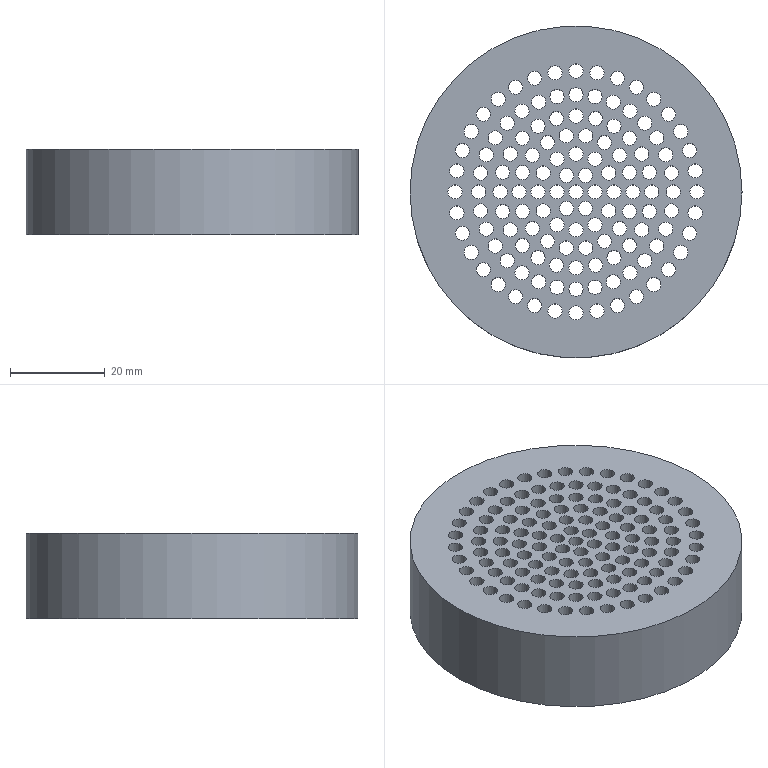NC program | NX | posted with a generic post | part box 70 x 70 x 18 mm
Whole program:
N10 G17 G21 G94 G90
(DRILLING_COPY_2 , TOOL : ZXZ)
N12 T01 M6
N14 G54
N16 G17 G0 G90 X-14.496 Y-14.496 S3000 M3
N18 G43 Z30. H1
N20 G94 G81 G98 Z-1. F250. R3.
N22 X-17.045 Y-11.389
N24 X-18.94 Y-7.845
N26 X-20.106 Y-3.999
N28 X-20.5 Y0.
N30 X-20.106 Y3.999
N32 X-18.94 Y7.845
N34 X-17.045 Y11.389
N36 X-14.496 Y14.496
N38 X-11.389 Y17.045
N40 X-7.845 Y18.94
N42 X-3.999 Y20.106
N44 X0. Y20.5
N46 X3.999 Y20.106
N48 X7.845 Y18.94
N50 X11.389 Y17.045
N52 X14.496 Y14.496
N54 X17.045 Y11.389
N56 X18.94 Y7.845
N58 X20.106 Y3.999
N60 X20.5 Y0.
N62 X20.106 Y-3.999
N64 X18.94 Y-7.845
N66 X17.045 Y-11.389
N68 X14.496 Y-14.496
N70 X11.389 Y-17.045
N72 X7.845 Y-18.94
N74 X3.999 Y-20.106
N76 X0. Y-20.5
N78 X-3.999 Y-20.106
N80 X-7.845 Y-18.94
N82 X-11.389 Y-17.045
N84 X-8. Y-13.856
N86 X-6. Y-10.392
N88 X-4. Y-6.928
N90 X-2. Y-3.464
N92 X-4. Y0.
N94 X-2. Y3.464
N96 X2.
N98 X4. Y6.928
N100 X6. Y10.392
N102 X9.193 Y7.713
N104 X6.928 Y4.
N106 X11.276 Y4.104
N108 X12. Y0.
N110 X11.276 Y-4.104
N112 X9.193 Y-7.713
N114 X6.928 Y-4.
N116 X8. Y0.
N118 X4.
N120 X0.
N122 X2. Y-3.464
N124 X4. Y-6.928
N126 X0. Y-8.
N128 X-2.084 Y-11.818
N130 X-4.141 Y-15.455
N132 X0. Y-16.
N134 X4.141 Y-15.455
N136 X2.084 Y-11.818
N138 X6. Y-10.392
N140 X8. Y-13.856
N142 X11.314 Y-11.314
N144 X13.856 Y-8.
N146 X15.455 Y-4.141
N148 X16. Y0.
N150 X15.455 Y4.141
N152 X13.856 Y8.
N154 X11.314 Y11.314
N156 X8. Y13.856
N158 X4.141 Y15.455
N160 X0. Y16.
N162 X-4.141 Y15.455
N164 X-8. Y13.856
N166 X-6. Y10.392
N168 X-2.084 Y11.818
N170 X2.084
N172 X0. Y8.
N174 X-4. Y6.928
N176 X-6.928 Y4.
N178 X-11.276 Y4.104
N180 X-9.193 Y7.713
N182 X-11.314 Y11.314
N184 X-13.856 Y8.
N186 X-15.455 Y4.141
N188 X-16. Y0.
N190 X-12.
N192 X-8.
N194 X-6.928 Y-4.
N196 X-9.193 Y-7.713
N198 X-11.276 Y-4.104
N200 X-15.455 Y-4.141
N202 X-13.856 Y-8.
N204 X-11.314 Y-11.314
N206 G80
N208 G0 X-11.314 Y-11.314 Z30.
N210 M5
(DRILLING_COPY_COPY , TOOL : 2.5ZT)
N212 T12 M6
N214 G54
N216 G17 G0 G90 X-14.496 Y-14.496 S2971 M3
N218 G43 Z30. H12
N220 G94 G83 G98 Z-19.751 F120. Q2. R3.
N222 X-17.045 Y-11.389
N224 X-18.94 Y-7.845
N226 X-20.106 Y-3.999
N228 X-20.5 Y0.
N230 X-20.106 Y3.999
N232 X-18.94 Y7.845
N234 X-17.045 Y11.389
N236 X-14.496 Y14.496
N238 X-11.389 Y17.045
N240 X-7.845 Y18.94
N242 X-3.999 Y20.106
N244 X0. Y20.5
N246 X3.999 Y20.106
N248 X7.845 Y18.94
N250 X11.389 Y17.045
N252 X14.496 Y14.496
N254 X17.045 Y11.389
N256 X18.94 Y7.845
N258 X20.106 Y3.999
N260 X20.5 Y0.
N262 X20.106 Y-3.999
N264 X18.94 Y-7.845
N266 X17.045 Y-11.389
N268 X14.496 Y-14.496
N270 X11.389 Y-17.045
N272 X7.845 Y-18.94
N274 X3.999 Y-20.106
N276 X0. Y-20.5
N278 X-3.999 Y-20.106
N280 X-7.845 Y-18.94
N282 X-11.389 Y-17.045
N284 X-8. Y-13.856
N286 X-6. Y-10.392
N288 X-4. Y-6.928
N290 X-2. Y-3.464
N292 X-4. Y0.
N294 X-2. Y3.464
N296 X2.
N298 X4. Y6.928
N300 X6. Y10.392
N302 X9.193 Y7.713
N304 X6.928 Y4.
N306 X11.276 Y4.104
N308 X12. Y0.
N310 X11.276 Y-4.104
N312 X9.193 Y-7.713
N314 X6.928 Y-4.
N316 X8. Y0.
N318 X4.
N320 X0.
N322 X2. Y-3.464
N324 X4. Y-6.928
N326 X0. Y-8.
N328 X-2.084 Y-11.818
N330 X-4.141 Y-15.455
N332 X0. Y-16.
N334 X4.141 Y-15.455
N336 X2.084 Y-11.818
N338 X6. Y-10.392
N340 X8. Y-13.856
N342 X11.314 Y-11.314
N344 X13.856 Y-8.
N346 X15.455 Y-4.141
N348 X16. Y0.
N350 X15.455 Y4.141
N352 X13.856 Y8.
N354 X11.314 Y11.314
N356 X8. Y13.856
N358 X4.141 Y15.455
N360 X0. Y16.
N362 X-4.141 Y15.455
N364 X-8. Y13.856
N366 X-6. Y10.392
N368 X-2.084 Y11.818
N370 X2.084
N372 X0. Y8.
N374 X-4. Y6.928
N376 X-6.928 Y4.
N378 X-11.276 Y4.104
N380 X-9.193 Y7.713
N382 X-11.314 Y11.314
N384 X-13.856 Y8.
N386 X-15.455 Y4.141
N388 X-16. Y0.
N390 X-12.
N392 X-8.
N394 X-6.928 Y-4.
N396 X-9.193 Y-7.713
N398 X-11.276 Y-4.104
N400 X-15.455 Y-4.141
N402 X-13.856 Y-8.
N404 X-11.314 Y-11.314
N406 G80
N408 G0 X-11.314 Y-11.314 Z30.
N410 M5
(DRILLING_COPY_1_COPY , TOOL : D6A45)
N412 T07 M6
N414 G54
N416 G17 G0 G90 X-14.496 Y-14.496 S3000 M3
N418 G43 Z30. H7
N420 G94 G81 G98 Z-1.35 F250. R3.
N422 X-17.045 Y-11.389
N424 X-18.94 Y-7.845
N426 X-20.106 Y-3.999
N428 X-20.5 Y0.
N430 X-20.106 Y3.999
N432 X-18.94 Y7.845
N434 X-17.045 Y11.389
N436 X-14.496 Y14.496
N438 X-11.389 Y17.045
N440 X-7.845 Y18.94
N442 X-3.999 Y20.106
N444 X0. Y20.5
N446 X3.999 Y20.106
N448 X7.845 Y18.94
N450 X11.389 Y17.045
N452 X14.496 Y14.496
N454 X17.045 Y11.389
N456 X18.94 Y7.845
N458 X20.106 Y3.999
N460 X20.5 Y0.
N462 X20.106 Y-3.999
N464 X18.94 Y-7.845
N466 X17.045 Y-11.389
N468 X14.496 Y-14.496
N470 X11.389 Y-17.045
N472 X7.845 Y-18.94
N474 X3.999 Y-20.106
N476 X0. Y-20.5
N478 X-3.999 Y-20.106
N480 X-7.845 Y-18.94
N482 X-11.389 Y-17.045
N484 X-8. Y-13.856
N486 X-6. Y-10.392
N488 X-4. Y-6.928
N490 X-2. Y-3.464
N492 X-4. Y0.
N494 X-2. Y3.464
N496 X2.
N498 X4. Y6.928
N500 X6. Y10.392
N502 X9.193 Y7.713
N504 X6.928 Y4.
N506 X11.276 Y4.104
N508 X12. Y0.
N510 X11.276 Y-4.104
N512 X9.193 Y-7.713
N514 X6.928 Y-4.
N516 X8. Y0.
N518 X4.
N520 X0.
N522 X2. Y-3.464
N524 X4. Y-6.928
N526 X0. Y-8.
N528 X-2.084 Y-11.818
N530 X-4.141 Y-15.455
N532 X0. Y-16.
N534 X4.141 Y-15.455
N536 X2.084 Y-11.818
N538 X6. Y-10.392
N540 X8. Y-13.856
N542 X11.314 Y-11.314
N544 X13.856 Y-8.
N546 X15.455 Y-4.141
N548 X16. Y0.
N550 X15.455 Y4.141
N552 X13.856 Y8.
N554 X11.314 Y11.314
N556 X8. Y13.856
N558 X4.141 Y15.455
N560 X0. Y16.
N562 X-4.141 Y15.455
N564 X-8. Y13.856
N566 X-6. Y10.392
N568 X-2.084 Y11.818
N570 X2.084
N572 X0. Y8.
N574 X-4. Y6.928
N576 X-6.928 Y4.
N578 X-11.276 Y4.104
N580 X-9.193 Y7.713
N582 X-11.314 Y11.314
N584 X-13.856 Y8.
N586 X-15.455 Y4.141
N588 X-16. Y0.
N590 X-12.
N592 X-8.
N594 X-6.928 Y-4.
N596 X-9.193 Y-7.713
N598 X-11.276 Y-4.104
N600 X-15.455 Y-4.141
N602 X-13.856 Y-8.
N604 X-11.314 Y-11.314
N606 G80
N608 G0 X-11.314 Y-11.314 Z30.
N610 M5
N612 M2